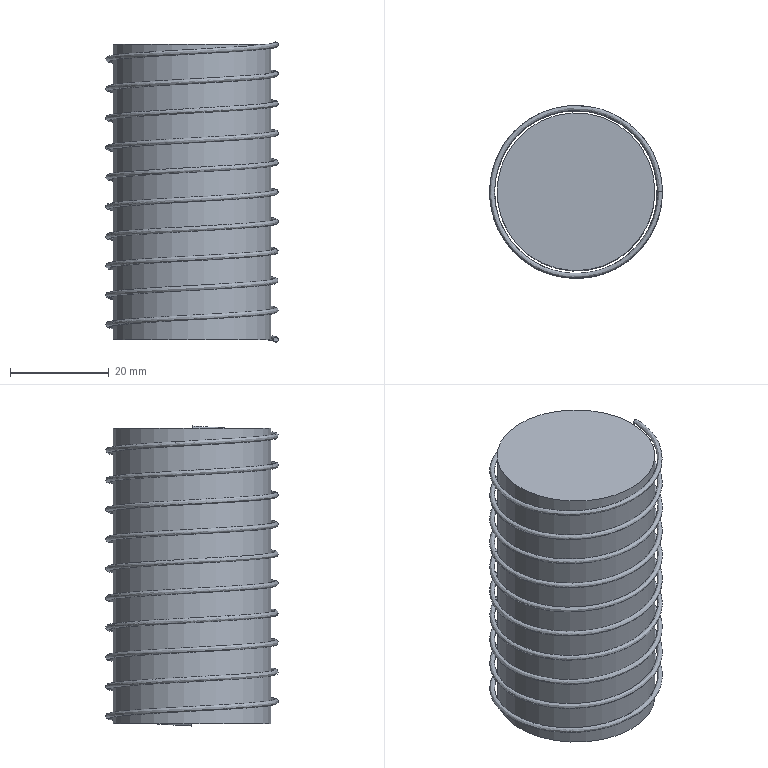Part | NX | features BREP 2 | 2 solids | 6 faces | box 35.014 x 35.015 x 60.848 mm | volume 48963 mm3 | plane 4 | cylinder 1 | spline 1 | commonest cylinder face diameters 32 x1